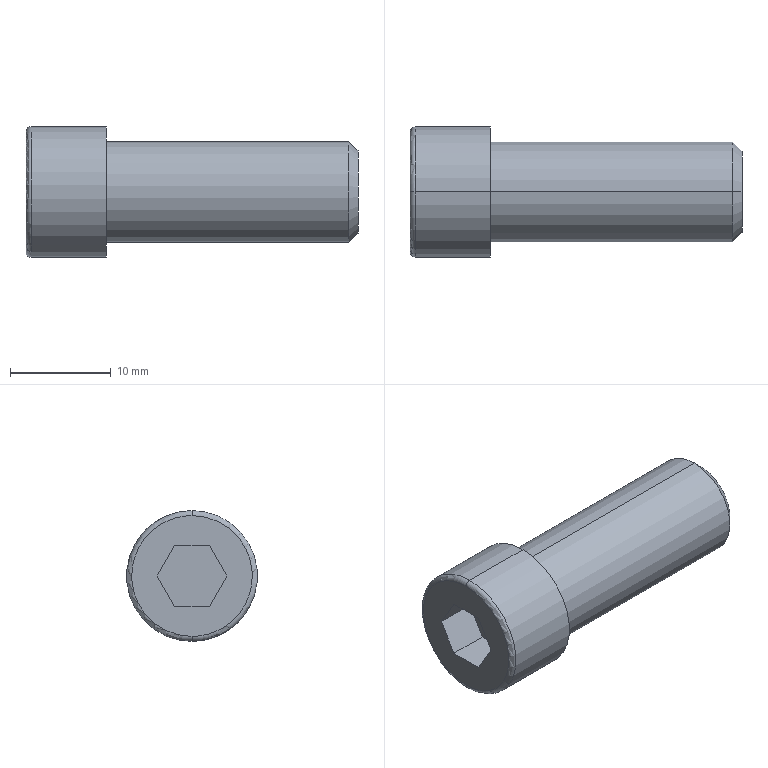Part | NX | features BREP 1 | 1 solid | 18 faces | box 33 x 13 x 13 mm | volume 2886 mm3 | plane 10 | cylinder 4 | torus 2 | cone 2 | commonest cylinder face diameters 10 x2 13 x2
STEP:
#1=CARTESIAN_POINT('',(-7.5,0.,6.5));
#2=VERTEX_POINT('',#1);
#3=CARTESIAN_POINT('',(-7.5,0.,-6.5));
#4=VERTEX_POINT('',#3);
#5=CARTESIAN_POINT('',(-7.5,0.,0.));
#6=DIRECTION('',(1.,0.,0.));
#7=DIRECTION('',(0.,0.,1.));
#8=AXIS2_PLACEMENT_3D('',#5,#6,#7);
#9=CIRCLE('',#8,6.5);
#10=EDGE_CURVE('',#2,#4,#9,.T.);
#11=ORIENTED_EDGE('',*,*,#10,.F.);
#12=CARTESIAN_POINT('',(-8.,0.,6.));
#13=VERTEX_POINT('',#12);
#14=CARTESIAN_POINT('',(-7.5,0.,6.));
#15=DIRECTION('',(0.,-1.,0.));
#16=DIRECTION('',(0.,0.,1.));
#17=AXIS2_PLACEMENT_3D('',#14,#15,#16);
#18=CIRCLE('',#17,0.5);
#19=EDGE_CURVE('',#2,#13,#18,.T.);
#20=ORIENTED_EDGE('',*,*,#19,.T.);
#21=CARTESIAN_POINT('',(-8.,0.,-6.));
#22=VERTEX_POINT('',#21);
#23=CARTESIAN_POINT('',(-8.,0.,6.));
#24=CARTESIAN_POINT('',(-8.,-12.,6.));
#25=CARTESIAN_POINT('',(-8.,-12.,-6.));
#26=CARTESIAN_POINT('',(-8.,0.,-6.));
#27=(BOUNDED_CURVE()B_SPLINE_CURVE(3,(#23,#24,#25,#26),.UNSPECIFIED.,.F.,.F.)B_SPLINE_CURVE_WITH_KNOTS((4,4),(0.5,1.),.UNSPECIFIED.)CURVE()GEOMETRIC_REPRESENTATION_ITEM()RATIONAL_B_SPLINE_CURVE((1.,0.3333,0.3333,1.))REPRESENTATION_ITEM(''));
#28=EDGE_CURVE('',#13,#22,#27,.T.);
#29=ORIENTED_EDGE('',*,*,#28,.T.);
#30=CARTESIAN_POINT('',(-7.5,0.,-6.));
#31=DIRECTION('',(0.,1.,0.));
#32=DIRECTION('',(0.,0.,-1.));
#33=AXIS2_PLACEMENT_3D('',#30,#31,#32);
#34=CIRCLE('',#33,0.5);
#35=EDGE_CURVE('',#4,#22,#34,.T.);
#36=ORIENTED_EDGE('',*,*,#35,.F.);
#37=EDGE_LOOP('',(#11,#20,#29,#36));
#38=FACE_BOUND('',#37,.T.);
#39=CARTESIAN_POINT('',(-7.5,0.,0.));
#40=DIRECTION('',(1.,0.,0.));
#41=DIRECTION('',(0.,0.,-1.));
#42=AXIS2_PLACEMENT_3D('',#39,#40,#41);
#43=TOROIDAL_SURFACE('',#42,6.,0.5);
#44=ADVANCED_FACE('',(#38),#43,.T.);
#45=CARTESIAN_POINT('',(24.08,0.,5.));
#46=VERTEX_POINT('',#45);
#47=CARTESIAN_POINT('',(24.08,0.,-5.));
#48=VERTEX_POINT('',#47);
#49=CARTESIAN_POINT('',(24.08,0.,0.));
#50=DIRECTION('',(-1.,0.,0.));
#51=DIRECTION('',(0.,0.,1.));
#52=AXIS2_PLACEMENT_3D('',#49,#50,#51);
#53=CIRCLE('',#52,5.);
#54=EDGE_CURVE('',#46,#48,#53,.T.);
#55=ORIENTED_EDGE('',*,*,#54,.T.);
#56=CARTESIAN_POINT('',(0.,0.,-5.));
#57=VERTEX_POINT('',#56);
#58=CARTESIAN_POINT('',(25.,0.,-5.));
#59=DIRECTION('',(-1.,0.,0.));
#60=VECTOR('',#59,1000.);
#61=LINE('',#58,#60);
#62=EDGE_CURVE('',#57,#48,#61,.F.);
#63=ORIENTED_EDGE('',*,*,#62,.F.);
#64=CARTESIAN_POINT('',(0.,0.,5.));
#65=VERTEX_POINT('',#64);
#66=CARTESIAN_POINT('',(0.,0.,0.));
#67=DIRECTION('',(1.,0.,0.));
#68=DIRECTION('',(0.,0.,1.));
#69=AXIS2_PLACEMENT_3D('',#66,#67,#68);
#70=CIRCLE('',#69,5.);
#71=EDGE_CURVE('',#57,#65,#70,.T.);
#72=ORIENTED_EDGE('',*,*,#71,.T.);
#73=CARTESIAN_POINT('',(25.,0.,5.));
#74=DIRECTION('',(-1.,0.,0.));
#75=VECTOR('',#74,1000.);
#76=LINE('',#73,#75);
#77=EDGE_CURVE('',#65,#46,#76,.F.);
#78=ORIENTED_EDGE('',*,*,#77,.T.);
#79=EDGE_LOOP('',(#55,#63,#72,#78));
#80=FACE_BOUND('',#79,.T.);
#81=CARTESIAN_POINT('',(25.,0.,0.));
#82=DIRECTION('',(-1.,0.,0.));
#83=DIRECTION('',(0.,0.,1.));
#84=AXIS2_PLACEMENT_3D('',#81,#82,#83);
#85=CYLINDRICAL_SURFACE('',#84,5.);
#86=ADVANCED_FACE('',(#80),#85,.T.);
#87=CARTESIAN_POINT('',(25.,0.,4.08));
#88=VERTEX_POINT('',#87);
#89=CARTESIAN_POINT('',(25.,0.,-4.08));
#90=VERTEX_POINT('',#89);
#91=CARTESIAN_POINT('',(25.,0.,0.));
#92=DIRECTION('',(-1.,0.,0.));
#93=DIRECTION('',(0.,0.,1.));
#94=AXIS2_PLACEMENT_3D('',#91,#92,#93);
#95=CIRCLE('',#94,4.08);
#96=EDGE_CURVE('',#88,#90,#95,.T.);
#97=ORIENTED_EDGE('',*,*,#96,.T.);
#98=CARTESIAN_POINT('',(24.08,0.,-5.));
#99=DIRECTION('',(-0.7071,0.,-0.7071));
#100=VECTOR('',#99,1000.);
#101=LINE('',#98,#100);
#102=EDGE_CURVE('',#48,#90,#101,.F.);
#103=ORIENTED_EDGE('',*,*,#102,.F.);
#104=ORIENTED_EDGE('',*,*,#54,.F.);
#105=CARTESIAN_POINT('',(24.08,0.,5.));
#106=DIRECTION('',(-0.7071,0.,0.7071));
#107=VECTOR('',#106,1000.);
#108=LINE('',#105,#107);
#109=EDGE_CURVE('',#46,#88,#108,.F.);
#110=ORIENTED_EDGE('',*,*,#109,.T.);
#111=EDGE_LOOP('',(#97,#103,#104,#110));
#112=FACE_BOUND('',#111,.T.);
#113=CARTESIAN_POINT('',(24.08,0.,0.));
#114=DIRECTION('',(-1.,0.,0.));
#115=DIRECTION('',(0.,0.,1.));
#116=AXIS2_PLACEMENT_3D('',#113,#114,#115);
#117=CONICAL_SURFACE('',#116,5.,0.7854);
#118=ADVANCED_FACE('',(#112),#117,.T.);
#119=CARTESIAN_POINT('',(0.,0.,6.5));
#120=VERTEX_POINT('',#119);
#121=CARTESIAN_POINT('',(0.,0.,-6.5));
#122=VERTEX_POINT('',#121);
#123=CARTESIAN_POINT('',(0.,0.,0.));
#124=DIRECTION('',(-1.,0.,0.));
#125=DIRECTION('',(0.,0.,1.));
#126=AXIS2_PLACEMENT_3D('',#123,#124,#125);
#127=CIRCLE('',#126,6.5);
#128=EDGE_CURVE('',#120,#122,#127,.T.);
#129=ORIENTED_EDGE('',*,*,#128,.T.);
#130=CARTESIAN_POINT('',(25.,0.,-6.5));
#131=DIRECTION('',(-1.,0.,0.));
#132=VECTOR('',#131,1000.);
#133=LINE('',#130,#132);
#134=EDGE_CURVE('',#4,#122,#133,.F.);
#135=ORIENTED_EDGE('',*,*,#134,.F.);
#136=CARTESIAN_POINT('',(-7.5,0.,0.));
#137=DIRECTION('',(1.,0.,0.));
#138=DIRECTION('',(0.,0.,1.));
#139=AXIS2_PLACEMENT_3D('',#136,#137,#138);
#140=CIRCLE('',#139,6.5);
#141=EDGE_CURVE('',#4,#2,#140,.T.);
#142=ORIENTED_EDGE('',*,*,#141,.T.);
#143=CARTESIAN_POINT('',(25.,0.,6.5));
#144=DIRECTION('',(-1.,0.,0.));
#145=VECTOR('',#144,1000.);
#146=LINE('',#143,#145);
#147=EDGE_CURVE('',#2,#120,#146,.F.);
#148=ORIENTED_EDGE('',*,*,#147,.T.);
#149=EDGE_LOOP('',(#129,#135,#142,#148));
#150=FACE_BOUND('',#149,.T.);
#151=CARTESIAN_POINT('',(25.,0.,0.));
#152=DIRECTION('',(-1.,0.,0.));
#153=DIRECTION('',(0.,0.,1.));
#154=AXIS2_PLACEMENT_3D('',#151,#152,#153);
#155=CYLINDRICAL_SURFACE('',#154,6.5);
#156=ADVANCED_FACE('',(#150),#155,.T.);
#157=ORIENTED_EDGE('',*,*,#62,.T.);
#158=CARTESIAN_POINT('',(24.08,0.,0.));
#159=DIRECTION('',(-1.,0.,0.));
#160=DIRECTION('',(0.,0.,1.));
#161=AXIS2_PLACEMENT_3D('',#158,#159,#160);
#162=CIRCLE('',#161,5.);
#163=EDGE_CURVE('',#48,#46,#162,.T.);
#164=ORIENTED_EDGE('',*,*,#163,.T.);
#165=ORIENTED_EDGE('',*,*,#77,.F.);
#166=CARTESIAN_POINT('',(0.,0.,0.));
#167=DIRECTION('',(1.,0.,0.));
#168=DIRECTION('',(0.,0.,1.));
#169=AXIS2_PLACEMENT_3D('',#166,#167,#168);
#170=CIRCLE('',#169,5.);
#171=EDGE_CURVE('',#65,#57,#170,.T.);
#172=ORIENTED_EDGE('',*,*,#171,.T.);
#173=EDGE_LOOP('',(#157,#164,#165,#172));
#174=FACE_BOUND('',#173,.T.);
#175=CARTESIAN_POINT('',(25.,0.,0.));
#176=DIRECTION('',(-1.,0.,0.));
#177=DIRECTION('',(0.,0.,1.));
#178=AXIS2_PLACEMENT_3D('',#175,#176,#177);
#179=CYLINDRICAL_SURFACE('',#178,5.);
#180=ADVANCED_FACE('',(#174),#179,.T.);
#181=ORIENTED_EDGE('',*,*,#128,.F.);
#182=CARTESIAN_POINT('',(0.,0.,0.));
#183=DIRECTION('',(-1.,0.,0.));
#184=DIRECTION('',(0.,0.,1.));
#185=AXIS2_PLACEMENT_3D('',#182,#183,#184);
#186=CIRCLE('',#185,6.5);
#187=EDGE_CURVE('',#122,#120,#186,.T.);
#188=ORIENTED_EDGE('',*,*,#187,.F.);
#189=EDGE_LOOP('',(#181,#188));
#190=FACE_BOUND('',#189,.T.);
#191=ORIENTED_EDGE('',*,*,#171,.F.);
#192=ORIENTED_EDGE('',*,*,#71,.F.);
#193=EDGE_LOOP('',(#191,#192));
#194=FACE_BOUND('',#193,.T.);
#195=CARTESIAN_POINT('',(0.,6.5,0.));
#196=DIRECTION('',(-1.,0.,0.));
#197=DIRECTION('',(0.,0.,1.));
#198=AXIS2_PLACEMENT_3D('',#195,#196,#197);
#199=PLANE('',#198);
#200=ADVANCED_FACE('',(#190,#194),#199,.F.);
#201=ORIENTED_EDGE('',*,*,#102,.T.);
#202=CARTESIAN_POINT('',(25.,0.,0.));
#203=DIRECTION('',(-1.,0.,0.));
#204=DIRECTION('',(0.,0.,1.));
#205=AXIS2_PLACEMENT_3D('',#202,#203,#204);
#206=CIRCLE('',#205,4.08);
#207=EDGE_CURVE('',#90,#88,#206,.T.);
#208=ORIENTED_EDGE('',*,*,#207,.T.);
#209=ORIENTED_EDGE('',*,*,#109,.F.);
#210=ORIENTED_EDGE('',*,*,#163,.F.);
#211=EDGE_LOOP('',(#201,#208,#209,#210));
#212=FACE_BOUND('',#211,.T.);
#213=CARTESIAN_POINT('',(24.08,0.,0.));
#214=DIRECTION('',(-1.,0.,0.));
#215=DIRECTION('',(0.,0.,1.));
#216=AXIS2_PLACEMENT_3D('',#213,#214,#215);
#217=CONICAL_SURFACE('',#216,5.,0.7854);
#218=ADVANCED_FACE('',(#212),#217,.T.);
#219=ORIENTED_EDGE('',*,*,#134,.T.);
#220=ORIENTED_EDGE('',*,*,#187,.T.);
#221=ORIENTED_EDGE('',*,*,#147,.F.);
#222=ORIENTED_EDGE('',*,*,#10,.T.);
#223=EDGE_LOOP('',(#219,#220,#221,#222));
#224=FACE_BOUND('',#223,.T.);
#225=CARTESIAN_POINT('',(25.,0.,0.));
#226=DIRECTION('',(-1.,0.,0.));
#227=DIRECTION('',(0.,0.,1.));
#228=AXIS2_PLACEMENT_3D('',#225,#226,#227);
#229=CYLINDRICAL_SURFACE('',#228,6.5);
#230=ADVANCED_FACE('',(#224),#229,.T.);
#231=ORIENTED_EDGE('',*,*,#96,.F.);
#232=ORIENTED_EDGE('',*,*,#207,.F.);
#233=EDGE_LOOP('',(#231,#232));
#234=FACE_BOUND('',#233,.T.);
#235=CARTESIAN_POINT('',(25.,4.08,0.));
#236=DIRECTION('',(-1.,0.,0.));
#237=DIRECTION('',(0.,0.,1.));
#238=AXIS2_PLACEMENT_3D('',#235,#236,#237);
#239=PLANE('',#238);
#240=ADVANCED_FACE('',(#234),#239,.F.);
#241=ORIENTED_EDGE('',*,*,#19,.F.);
#242=ORIENTED_EDGE('',*,*,#141,.F.);
#243=ORIENTED_EDGE('',*,*,#35,.T.);
#244=CARTESIAN_POINT('',(-8.,0.,-6.));
#245=CARTESIAN_POINT('',(-8.,12.,-6.));
#246=CARTESIAN_POINT('',(-8.,12.,6.));
#247=CARTESIAN_POINT('',(-8.,0.,6.));
#248=(BOUNDED_CURVE()B_SPLINE_CURVE(3,(#244,#245,#246,#247),.UNSPECIFIED.,.F.,.F.)B_SPLINE_CURVE_WITH_KNOTS((4,4),(0.,0.5),.UNSPECIFIED.)CURVE()GEOMETRIC_REPRESENTATION_ITEM()RATIONAL_B_SPLINE_CURVE((1.,0.3333,0.3333,1.))REPRESENTATION_ITEM(''));
#249=EDGE_CURVE('',#22,#13,#248,.T.);
#250=ORIENTED_EDGE('',*,*,#249,.T.);
#251=EDGE_LOOP('',(#241,#242,#243,#250));
#252=FACE_BOUND('',#251,.T.);
#253=CARTESIAN_POINT('',(-7.5,0.,0.));
#254=DIRECTION('',(1.,0.,0.));
#255=DIRECTION('',(0.,0.,-1.));
#256=AXIS2_PLACEMENT_3D('',#253,#254,#255);
#257=TOROIDAL_SURFACE('',#256,6.,0.5);
#258=ADVANCED_FACE('',(#252),#257,.T.);
#259=ORIENTED_EDGE('',*,*,#249,.F.);
#260=ORIENTED_EDGE('',*,*,#28,.F.);
#261=EDGE_LOOP('',(#259,#260));
#262=FACE_BOUND('',#261,.T.);
#263=CARTESIAN_POINT('',(-8.,-3.464,0.));
#264=VERTEX_POINT('',#263);
#265=CARTESIAN_POINT('',(-8.,-1.732,3.));
#266=VERTEX_POINT('',#265);
#267=CARTESIAN_POINT('',(-8.,-3.464,0.));
#268=DIRECTION('',(0.,0.5,0.866));
#269=VECTOR('',#268,1000.);
#270=LINE('',#267,#269);
#271=EDGE_CURVE('',#264,#266,#270,.T.);
#272=ORIENTED_EDGE('',*,*,#271,.F.);
#273=CARTESIAN_POINT('',(-8.,-1.732,-3.));
#274=VERTEX_POINT('',#273);
#275=CARTESIAN_POINT('',(-8.,-1.732,-3.));
#276=DIRECTION('',(0.,-0.5,0.866));
#277=VECTOR('',#276,1000.);
#278=LINE('',#275,#277);
#279=EDGE_CURVE('',#274,#264,#278,.T.);
#280=ORIENTED_EDGE('',*,*,#279,.F.);
#281=CARTESIAN_POINT('',(-8.,1.732,-3.));
#282=VERTEX_POINT('',#281);
#283=CARTESIAN_POINT('',(-8.,0.,-3.));
#284=DIRECTION('',(0.,-1.,0.));
#285=VECTOR('',#284,1000.);
#286=LINE('',#283,#285);
#287=EDGE_CURVE('',#282,#274,#286,.T.);
#288=ORIENTED_EDGE('',*,*,#287,.F.);
#289=CARTESIAN_POINT('',(-8.,3.464,0.));
#290=VERTEX_POINT('',#289);
#291=CARTESIAN_POINT('',(-8.,3.464,0.));
#292=DIRECTION('',(0.,-0.5,-0.866));
#293=VECTOR('',#292,1000.);
#294=LINE('',#291,#293);
#295=EDGE_CURVE('',#290,#282,#294,.T.);
#296=ORIENTED_EDGE('',*,*,#295,.F.);
#297=CARTESIAN_POINT('',(-8.,1.732,3.));
#298=VERTEX_POINT('',#297);
#299=CARTESIAN_POINT('',(-8.,1.732,3.));
#300=DIRECTION('',(0.,0.5,-0.866));
#301=VECTOR('',#300,1000.);
#302=LINE('',#299,#301);
#303=EDGE_CURVE('',#298,#290,#302,.T.);
#304=ORIENTED_EDGE('',*,*,#303,.F.);
#305=CARTESIAN_POINT('',(-8.,0.,3.));
#306=DIRECTION('',(0.,1.,0.));
#307=VECTOR('',#306,1000.);
#308=LINE('',#305,#307);
#309=EDGE_CURVE('',#266,#298,#308,.T.);
#310=ORIENTED_EDGE('',*,*,#309,.F.);
#311=EDGE_LOOP('',(#272,#280,#288,#296,#304,#310));
#312=FACE_BOUND('',#311,.T.);
#313=CARTESIAN_POINT('',(-8.,0.,0.));
#314=DIRECTION('',(1.,0.,0.));
#315=DIRECTION('',(0.,1.,0.));
#316=AXIS2_PLACEMENT_3D('',#313,#314,#315);
#317=PLANE('',#316);
#318=ADVANCED_FACE('',(#262,#312),#317,.F.);
#319=CARTESIAN_POINT('',(-4.,1.732,3.));
#320=VERTEX_POINT('',#319);
#321=CARTESIAN_POINT('',(-4.,-1.732,3.));
#322=VERTEX_POINT('',#321);
#323=CARTESIAN_POINT('',(-4.,1.732,3.));
#324=DIRECTION('',(0.,-1.,0.));
#325=VECTOR('',#324,1000.);
#326=LINE('',#323,#325);
#327=EDGE_CURVE('',#320,#322,#326,.T.);
#328=ORIENTED_EDGE('',*,*,#327,.T.);
#329=CARTESIAN_POINT('',(-4.,-1.732,3.));
#330=DIRECTION('',(-1.,0.,0.));
#331=VECTOR('',#330,1000.);
#332=LINE('',#329,#331);
#333=EDGE_CURVE('',#322,#266,#332,.T.);
#334=ORIENTED_EDGE('',*,*,#333,.T.);
#335=ORIENTED_EDGE('',*,*,#309,.T.);
#336=CARTESIAN_POINT('',(-4.,1.732,3.));
#337=DIRECTION('',(1.,0.,0.));
#338=VECTOR('',#337,1000.);
#339=LINE('',#336,#338);
#340=EDGE_CURVE('',#298,#320,#339,.T.);
#341=ORIENTED_EDGE('',*,*,#340,.T.);
#342=EDGE_LOOP('',(#328,#334,#335,#341));
#343=FACE_BOUND('',#342,.T.);
#344=CARTESIAN_POINT('',(-4.,1.732,3.));
#345=DIRECTION('',(0.,0.,-1.));
#346=DIRECTION('',(0.,-1.,0.));
#347=AXIS2_PLACEMENT_3D('',#344,#345,#346);
#348=PLANE('',#347);
#349=ADVANCED_FACE('',(#343),#348,.T.);
#350=CARTESIAN_POINT('',(-4.,-3.464,0.));
#351=VERTEX_POINT('',#350);
#352=CARTESIAN_POINT('',(-4.,-1.732,3.));
#353=DIRECTION('',(0.,-0.5,-0.866));
#354=VECTOR('',#353,1000.);
#355=LINE('',#352,#354);
#356=EDGE_CURVE('',#322,#351,#355,.T.);
#357=ORIENTED_EDGE('',*,*,#356,.T.);
#358=CARTESIAN_POINT('',(-4.,-3.464,0.));
#359=DIRECTION('',(-1.,0.,0.));
#360=VECTOR('',#359,1000.);
#361=LINE('',#358,#360);
#362=EDGE_CURVE('',#351,#264,#361,.T.);
#363=ORIENTED_EDGE('',*,*,#362,.T.);
#364=ORIENTED_EDGE('',*,*,#271,.T.);
#365=ORIENTED_EDGE('',*,*,#333,.F.);
#366=EDGE_LOOP('',(#357,#363,#364,#365));
#367=FACE_BOUND('',#366,.T.);
#368=CARTESIAN_POINT('',(-4.,-1.732,3.));
#369=DIRECTION('',(0.,0.866,-0.5));
#370=DIRECTION('',(-1.,0.,0.));
#371=AXIS2_PLACEMENT_3D('',#368,#369,#370);
#372=PLANE('',#371);
#373=ADVANCED_FACE('',(#367),#372,.T.);
#374=CARTESIAN_POINT('',(-4.,-1.732,-3.));
#375=VERTEX_POINT('',#374);
#376=CARTESIAN_POINT('',(-4.,-3.464,0.));
#377=DIRECTION('',(0.,0.5,-0.866));
#378=VECTOR('',#377,1000.);
#379=LINE('',#376,#378);
#380=EDGE_CURVE('',#351,#375,#379,.T.);
#381=ORIENTED_EDGE('',*,*,#380,.T.);
#382=CARTESIAN_POINT('',(-4.,-1.732,-3.));
#383=DIRECTION('',(-1.,0.,0.));
#384=VECTOR('',#383,1000.);
#385=LINE('',#382,#384);
#386=EDGE_CURVE('',#375,#274,#385,.T.);
#387=ORIENTED_EDGE('',*,*,#386,.T.);
#388=ORIENTED_EDGE('',*,*,#279,.T.);
#389=ORIENTED_EDGE('',*,*,#362,.F.);
#390=EDGE_LOOP('',(#381,#387,#388,#389));
#391=FACE_BOUND('',#390,.T.);
#392=CARTESIAN_POINT('',(-4.,-3.464,0.));
#393=DIRECTION('',(0.,0.866,0.5));
#394=DIRECTION('',(1.,0.,0.));
#395=AXIS2_PLACEMENT_3D('',#392,#393,#394);
#396=PLANE('',#395);
#397=ADVANCED_FACE('',(#391),#396,.T.);
#398=CARTESIAN_POINT('',(-4.,1.732,-3.));
#399=VERTEX_POINT('',#398);
#400=CARTESIAN_POINT('',(-4.,-1.732,-3.));
#401=DIRECTION('',(0.,1.,0.));
#402=VECTOR('',#401,1000.);
#403=LINE('',#400,#402);
#404=EDGE_CURVE('',#375,#399,#403,.T.);
#405=ORIENTED_EDGE('',*,*,#404,.T.);
#406=CARTESIAN_POINT('',(-4.,1.732,-3.));
#407=DIRECTION('',(-1.,0.,0.));
#408=VECTOR('',#407,1000.);
#409=LINE('',#406,#408);
#410=EDGE_CURVE('',#399,#282,#409,.T.);
#411=ORIENTED_EDGE('',*,*,#410,.T.);
#412=ORIENTED_EDGE('',*,*,#287,.T.);
#413=ORIENTED_EDGE('',*,*,#386,.F.);
#414=EDGE_LOOP('',(#405,#411,#412,#413));
#415=FACE_BOUND('',#414,.T.);
#416=CARTESIAN_POINT('',(-4.,-1.732,-3.));
#417=DIRECTION('',(0.,0.,1.));
#418=DIRECTION('',(1.,0.,0.));
#419=AXIS2_PLACEMENT_3D('',#416,#417,#418);
#420=PLANE('',#419);
#421=ADVANCED_FACE('',(#415),#420,.T.);
#422=CARTESIAN_POINT('',(-4.,3.464,0.));
#423=VERTEX_POINT('',#422);
#424=CARTESIAN_POINT('',(-4.,1.732,-3.));
#425=DIRECTION('',(0.,0.5,0.866));
#426=VECTOR('',#425,1000.);
#427=LINE('',#424,#426);
#428=EDGE_CURVE('',#399,#423,#427,.T.);
#429=ORIENTED_EDGE('',*,*,#428,.T.);
#430=CARTESIAN_POINT('',(-4.,3.464,0.));
#431=DIRECTION('',(-1.,0.,0.));
#432=VECTOR('',#431,1000.);
#433=LINE('',#430,#432);
#434=EDGE_CURVE('',#423,#290,#433,.T.);
#435=ORIENTED_EDGE('',*,*,#434,.T.);
#436=ORIENTED_EDGE('',*,*,#295,.T.);
#437=ORIENTED_EDGE('',*,*,#410,.F.);
#438=EDGE_LOOP('',(#429,#435,#436,#437));
#439=FACE_BOUND('',#438,.T.);
#440=CARTESIAN_POINT('',(-4.,1.732,-3.));
#441=DIRECTION('',(0.,-0.866,0.5));
#442=DIRECTION('',(-1.,0.,0.));
#443=AXIS2_PLACEMENT_3D('',#440,#441,#442);
#444=PLANE('',#443);
#445=ADVANCED_FACE('',(#439),#444,.T.);
#446=CARTESIAN_POINT('',(-4.,3.464,0.));
#447=DIRECTION('',(0.,-0.5,0.866));
#448=VECTOR('',#447,1000.);
#449=LINE('',#446,#448);
#450=EDGE_CURVE('',#423,#320,#449,.T.);
#451=ORIENTED_EDGE('',*,*,#450,.T.);
#452=ORIENTED_EDGE('',*,*,#340,.F.);
#453=ORIENTED_EDGE('',*,*,#303,.T.);
#454=ORIENTED_EDGE('',*,*,#434,.F.);
#455=EDGE_LOOP('',(#451,#452,#453,#454));
#456=FACE_BOUND('',#455,.T.);
#457=CARTESIAN_POINT('',(-4.,3.464,0.));
#458=DIRECTION('',(0.,-0.866,-0.5));
#459=DIRECTION('',(0.,0.5,-0.866));
#460=AXIS2_PLACEMENT_3D('',#457,#458,#459);
#461=PLANE('',#460);
#462=ADVANCED_FACE('',(#456),#461,.T.);
#463=ORIENTED_EDGE('',*,*,#450,.F.);
#464=ORIENTED_EDGE('',*,*,#428,.F.);
#465=ORIENTED_EDGE('',*,*,#404,.F.);
#466=ORIENTED_EDGE('',*,*,#380,.F.);
#467=ORIENTED_EDGE('',*,*,#356,.F.);
#468=ORIENTED_EDGE('',*,*,#327,.F.);
#469=EDGE_LOOP('',(#463,#464,#465,#466,#467,#468));
#470=FACE_BOUND('',#469,.T.);
#471=CARTESIAN_POINT('',(-4.,0.,0.));
#472=DIRECTION('',(1.,0.,0.));
#473=DIRECTION('',(0.,1.,0.));
#474=AXIS2_PLACEMENT_3D('',#471,#472,#473);
#475=PLANE('',#474);
#476=ADVANCED_FACE('',(#470),#475,.F.);
#477=CLOSED_SHELL('',(#44,#86,#118,#156,#180,#200,#218,#230,#240,#258,#318,#349,#373,#397,#421,#445,#462,#476));
#478=MANIFOLD_SOLID_BREP('',#477);
#479=(LENGTH_UNIT()NAMED_UNIT(*)SI_UNIT(.MILLI.,.METRE.));
#480=UNCERTAINTY_MEASURE_WITH_UNIT(LENGTH_MEASURE(0.00001),#479,'','');
#481=(NAMED_UNIT(*)PLANE_ANGLE_UNIT()SI_UNIT($,.RADIAN.));
#482=(NAMED_UNIT(*)SI_UNIT($,.STERADIAN.)SOLID_ANGLE_UNIT());
#483=(GEOMETRIC_REPRESENTATION_CONTEXT(3)GLOBAL_UNCERTAINTY_ASSIGNED_CONTEXT((#480))GLOBAL_UNIT_ASSIGNED_CONTEXT((#479,#481,#482))REPRESENTATION_CONTEXT('',''));
#484=ADVANCED_BREP_SHAPE_REPRESENTATION('',(#478),#483);